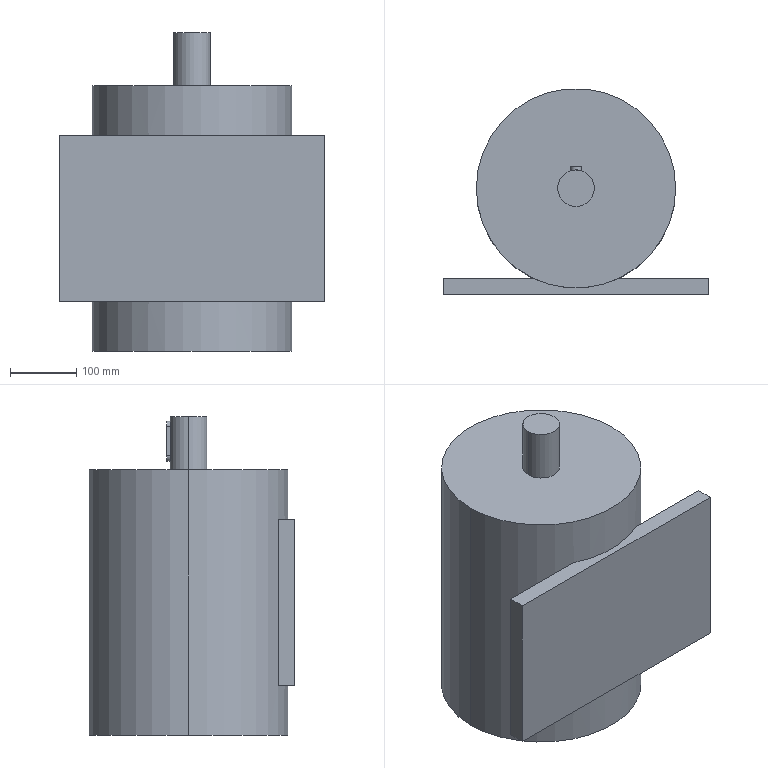Part | STEP file | Motor | 1 solid | 20 faces | box 400 x 310 x 480 mm | volume 30638928 mm3 | plane 13 | cylinder 7 | commonest cylinder face diameters 16 x3 55 x2 300 x2